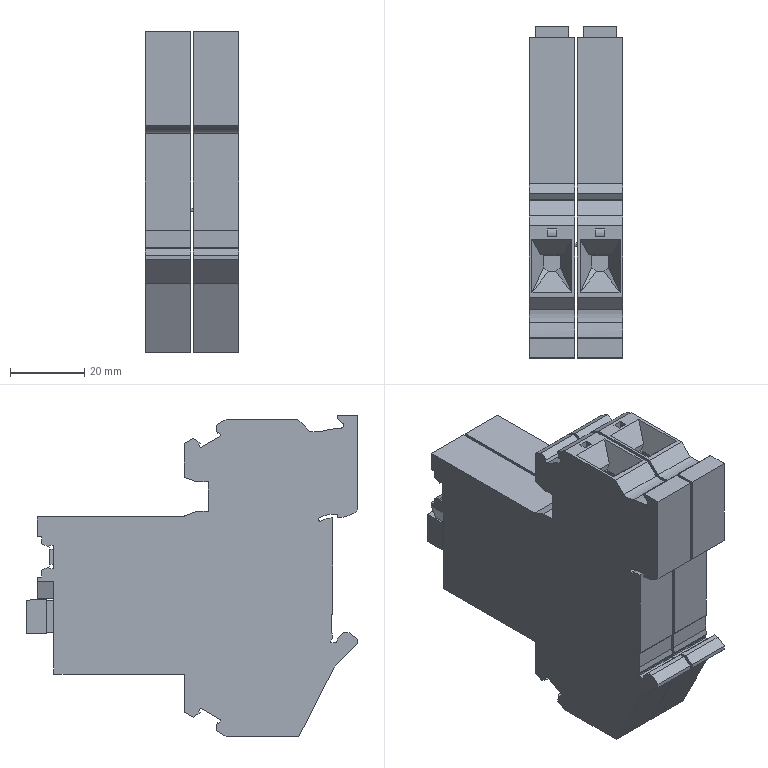Part | SolidWorks | features BaseBody 1 | 1 solid | 422 faces | box 25.3 x 89.537 x 86.5 mm | volume 117361 mm3 | plane 353 | cylinder 50 | spline 19 | commonest cylinder face diameters 4.82 x8 1 x6 0.8 x4 1.5 x4 4 x4 1.8 x2